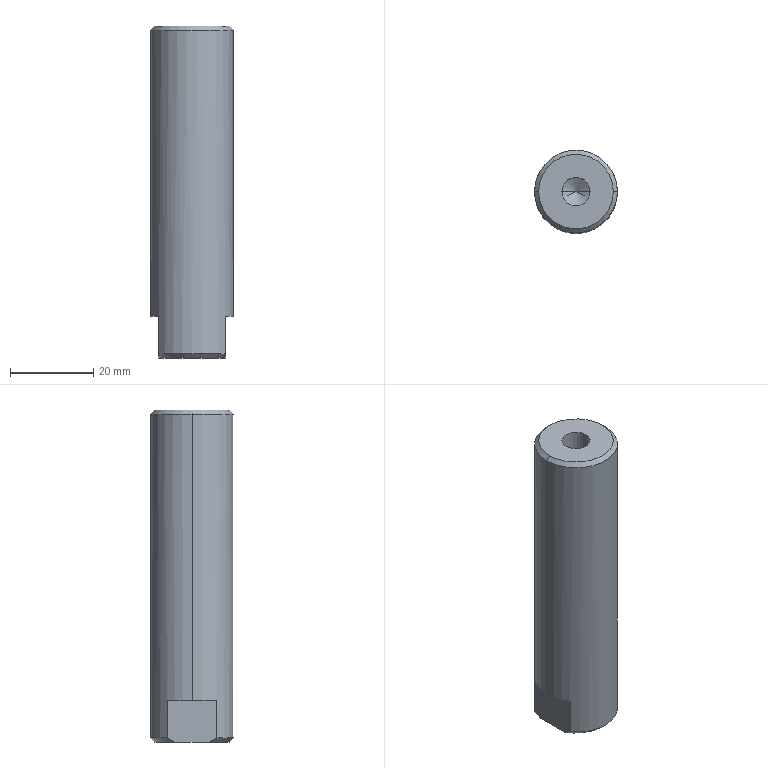Part | STEP file | 1 solid | 16 faces | box 20 x 20 x 80 mm | volume 24015 mm3 | cone 6 | plane 6 | cylinder 4 | commonest cylinder face diameters 6.8 x2 20 x2
STEP:
#1=CARTESIAN_POINT('',(0.,0.,0.));
#2=DIRECTION('',(0.,0.,1.));
#3=DIRECTION('',(1.,0.,0.));
#4=AXIS2_PLACEMENT_3D('',#1,#2,#3);
#5=CARTESIAN_POINT('',(3.4,0.,60.25));
#6=VERTEX_POINT('',#5);
#7=CARTESIAN_POINT('',(3.4,0.,80.));
#8=VERTEX_POINT('',#7);
#9=CARTESIAN_POINT('',(3.4,0.,80.));
#10=DIRECTION('',(0.,0.,1.));
#11=VECTOR('',#10,1.);
#12=LINE('',#9,#11);
#13=CARTESIAN_POINT('',(0.,0.,80.));
#14=DIRECTION('',(0.,0.,1.));
#15=DIRECTION('',(1.,0.,0.));
#16=AXIS2_PLACEMENT_3D('',#13,#14,#15);
#17=CYLINDRICAL_SURFACE('',#16,3.4);
#18=CARTESIAN_POINT('',(6.283,0.));
#19=DIRECTION('',(0.,1.));
#20=VECTOR('',#19,1.);
#21=LINE('',#18,#20);
#22=(GEOMETRIC_REPRESENTATION_CONTEXT(2)PARAMETRIC_REPRESENTATION_CONTEXT()REPRESENTATION_CONTEXT('',''));
#23=DEFINITIONAL_REPRESENTATION('',(#21),#22);
#24=PCURVE('',#17,#23);
#25=CARTESIAN_POINT('',(0.,0.,80.));
#26=DIRECTION('',(0.,0.,1.));
#27=DIRECTION('',(1.,0.,0.));
#28=AXIS2_PLACEMENT_3D('',#25,#26,#27);
#29=CYLINDRICAL_SURFACE('',#28,3.4);
#30=CARTESIAN_POINT('',(0.,0.));
#31=DIRECTION('',(0.,1.));
#32=VECTOR('',#31,1.);
#33=LINE('',#30,#32);
#34=(GEOMETRIC_REPRESENTATION_CONTEXT(2)PARAMETRIC_REPRESENTATION_CONTEXT()REPRESENTATION_CONTEXT('',''));
#35=DEFINITIONAL_REPRESENTATION('',(#33),#34);
#36=PCURVE('',#29,#35);
#37=SURFACE_CURVE('',#12,(#24,#36),.PCURVE_S1.);
#38=EDGE_CURVE('',#6,#8,#37,.T.);
#39=ORIENTED_EDGE('',*,*,#38,.T.);
#40=CARTESIAN_POINT('',(-3.4,0.,80.));
#41=VERTEX_POINT('',#40);
#42=CARTESIAN_POINT('',(0.,0.,80.));
#43=DIRECTION('',(0.,0.,1.));
#44=DIRECTION('',(1.,0.,0.));
#45=AXIS2_PLACEMENT_3D('',#42,#43,#44);
#46=CIRCLE('',#45,3.4);
#47=CARTESIAN_POINT('',(0.,0.));
#48=DIRECTION('',(1.,0.));
#49=VECTOR('',#48,1.);
#50=LINE('',#47,#49);
#51=(GEOMETRIC_REPRESENTATION_CONTEXT(2)PARAMETRIC_REPRESENTATION_CONTEXT()REPRESENTATION_CONTEXT('',''));
#52=DEFINITIONAL_REPRESENTATION('',(#50),#51);
#53=PCURVE('',#17,#52);
#54=CARTESIAN_POINT('',(0.,0.,80.));
#55=DIRECTION('',(0.,0.,1.));
#56=DIRECTION('',(1.,0.,0.));
#57=AXIS2_PLACEMENT_3D('',#54,#55,#56);
#58=PLANE('',#57);
#59=CARTESIAN_POINT('',(0.,0.));
#60=DIRECTION('',(1.,0.));
#61=AXIS2_PLACEMENT_2D('',#59,#60);
#62=CIRCLE('',#61,3.4);
#63=(GEOMETRIC_REPRESENTATION_CONTEXT(2)PARAMETRIC_REPRESENTATION_CONTEXT()REPRESENTATION_CONTEXT('',''));
#64=DEFINITIONAL_REPRESENTATION('',(#62),#63);
#65=PCURVE('',#58,#64);
#66=SURFACE_CURVE('',#46,(#53,#65),.PCURVE_S1.);
#67=EDGE_CURVE('',#41,#8,#66,.T.);
#68=ORIENTED_EDGE('',*,*,#67,.F.);
#69=CARTESIAN_POINT('',(-3.4,0.,60.25));
#70=VERTEX_POINT('',#69);
#71=CARTESIAN_POINT('',(-3.4,0.,80.));
#72=DIRECTION('',(0.,0.,1.));
#73=VECTOR('',#72,1.);
#74=LINE('',#71,#73);
#75=CARTESIAN_POINT('',(3.142,0.));
#76=DIRECTION('',(0.,1.));
#77=VECTOR('',#76,1.);
#78=LINE('',#75,#77);
#79=(GEOMETRIC_REPRESENTATION_CONTEXT(2)PARAMETRIC_REPRESENTATION_CONTEXT()REPRESENTATION_CONTEXT('',''));
#80=DEFINITIONAL_REPRESENTATION('',(#78),#79);
#81=PCURVE('',#17,#80);
#82=CARTESIAN_POINT('',(3.142,0.));
#83=DIRECTION('',(0.,1.));
#84=VECTOR('',#83,1.);
#85=LINE('',#82,#84);
#86=(GEOMETRIC_REPRESENTATION_CONTEXT(2)PARAMETRIC_REPRESENTATION_CONTEXT()REPRESENTATION_CONTEXT('',''));
#87=DEFINITIONAL_REPRESENTATION('',(#85),#86);
#88=PCURVE('',#29,#87);
#89=SURFACE_CURVE('',#74,(#81,#88),.PCURVE_S1.);
#90=EDGE_CURVE('',#70,#41,#89,.T.);
#91=ORIENTED_EDGE('',*,*,#90,.F.);
#92=CARTESIAN_POINT('',(0.,0.,60.25));
#93=DIRECTION('',(0.,0.,1.));
#94=DIRECTION('',(1.,0.,0.));
#95=AXIS2_PLACEMENT_3D('',#92,#93,#94);
#96=CIRCLE('',#95,3.4);
#97=CARTESIAN_POINT('',(0.,-19.75));
#98=DIRECTION('',(1.,0.));
#99=VECTOR('',#98,1.);
#100=LINE('',#97,#99);
#101=(GEOMETRIC_REPRESENTATION_CONTEXT(2)PARAMETRIC_REPRESENTATION_CONTEXT()REPRESENTATION_CONTEXT('',''));
#102=DEFINITIONAL_REPRESENTATION('',(#100),#101);
#103=PCURVE('',#17,#102);
#104=CARTESIAN_POINT('',(0.,0.,60.25));
#105=DIRECTION('',(0.,0.,1.));
#106=DIRECTION('',(1.,0.,0.));
#107=AXIS2_PLACEMENT_3D('',#104,#105,#106);
#108=CONICAL_SURFACE('',#107,3.4,1.03);
#109=CARTESIAN_POINT('',(0.,0.));
#110=DIRECTION('',(1.,0.));
#111=VECTOR('',#110,1.);
#112=LINE('',#109,#111);
#113=(GEOMETRIC_REPRESENTATION_CONTEXT(2)PARAMETRIC_REPRESENTATION_CONTEXT()REPRESENTATION_CONTEXT('',''));
#114=DEFINITIONAL_REPRESENTATION('',(#112),#113);
#115=PCURVE('',#108,#114);
#116=SURFACE_CURVE('',#96,(#103,#115),.PCURVE_S1.);
#117=EDGE_CURVE('',#70,#6,#116,.T.);
#118=ORIENTED_EDGE('',*,*,#117,.T.);
#119=EDGE_LOOP('',(#39,#68,#91,#118));
#120=FACE_BOUND('',#119,.F.);
#121=ADVANCED_FACE('',(#120),#17,.F.);
#122=ORIENTED_EDGE('',*,*,#117,.F.);
#123=CARTESIAN_POINT('',(0.,0.,58.207));
#124=VERTEX_POINT('',#123);
#125=CARTESIAN_POINT('',(-3.4,0.,60.25));
#126=DIRECTION('',(-0.8572,0.,0.515));
#127=VECTOR('',#126,1.);
#128=LINE('',#125,#127);
#129=CARTESIAN_POINT('',(3.142,0.));
#130=DIRECTION('',(0.,1.));
#131=VECTOR('',#130,1.);
#132=LINE('',#129,#131);
#133=(GEOMETRIC_REPRESENTATION_CONTEXT(2)PARAMETRIC_REPRESENTATION_CONTEXT()REPRESENTATION_CONTEXT('',''));
#134=DEFINITIONAL_REPRESENTATION('',(#132),#133);
#135=PCURVE('',#108,#134);
#136=CARTESIAN_POINT('',(0.,0.,60.25));
#137=DIRECTION('',(0.,0.,1.));
#138=DIRECTION('',(1.,0.,0.));
#139=AXIS2_PLACEMENT_3D('',#136,#137,#138);
#140=CONICAL_SURFACE('',#139,3.4,1.03);
#141=CARTESIAN_POINT('',(3.142,0.));
#142=DIRECTION('',(0.,1.));
#143=VECTOR('',#142,1.);
#144=LINE('',#141,#143);
#145=(GEOMETRIC_REPRESENTATION_CONTEXT(2)PARAMETRIC_REPRESENTATION_CONTEXT()REPRESENTATION_CONTEXT('',''));
#146=DEFINITIONAL_REPRESENTATION('',(#144),#145);
#147=PCURVE('',#140,#146);
#148=SURFACE_CURVE('',#128,(#135,#147),.PCURVE_S1.);
#149=EDGE_CURVE('',#124,#70,#148,.T.);
#150=ORIENTED_EDGE('',*,*,#149,.F.);
#151=CARTESIAN_POINT('',(3.4,0.,60.25));
#152=DIRECTION('',(0.8572,0.,0.515));
#153=VECTOR('',#152,1.);
#154=LINE('',#151,#153);
#155=CARTESIAN_POINT('',(6.283,0.));
#156=DIRECTION('',(0.,1.));
#157=VECTOR('',#156,1.);
#158=LINE('',#155,#157);
#159=(GEOMETRIC_REPRESENTATION_CONTEXT(2)PARAMETRIC_REPRESENTATION_CONTEXT()REPRESENTATION_CONTEXT('',''));
#160=DEFINITIONAL_REPRESENTATION('',(#158),#159);
#161=PCURVE('',#108,#160);
#162=CARTESIAN_POINT('',(0.,0.));
#163=DIRECTION('',(0.,1.));
#164=VECTOR('',#163,1.);
#165=LINE('',#162,#164);
#166=(GEOMETRIC_REPRESENTATION_CONTEXT(2)PARAMETRIC_REPRESENTATION_CONTEXT()REPRESENTATION_CONTEXT('',''));
#167=DEFINITIONAL_REPRESENTATION('',(#165),#166);
#168=PCURVE('',#140,#167);
#169=SURFACE_CURVE('',#154,(#161,#168),.PCURVE_S1.);
#170=EDGE_CURVE('',#124,#6,#169,.T.);
#171=ORIENTED_EDGE('',*,*,#170,.T.);
#172=EDGE_LOOP('',(#122,#150,#171));
#173=FACE_BOUND('',#172,.F.);
#174=ADVANCED_FACE('',(#173),#108,.F.);
#175=CARTESIAN_POINT('',(9.,0.,80.));
#176=VERTEX_POINT('',#175);
#177=CARTESIAN_POINT('',(-9.,0.,80.));
#178=VERTEX_POINT('',#177);
#179=CARTESIAN_POINT('',(0.,0.,80.));
#180=DIRECTION('',(0.,0.,1.));
#181=DIRECTION('',(1.,0.,0.));
#182=AXIS2_PLACEMENT_3D('',#179,#180,#181);
#183=CIRCLE('',#182,9.);
#184=CARTESIAN_POINT('',(0.,0.,80.));
#185=DIRECTION('',(0.,0.,-1.));
#186=DIRECTION('',(-1.,0.,0.));
#187=AXIS2_PLACEMENT_3D('',#184,#185,#186);
#188=CONICAL_SURFACE('',#187,9.,0.7854);
#189=CARTESIAN_POINT('',(3.142,0.));
#190=DIRECTION('',(-1.,0.));
#191=VECTOR('',#190,1.);
#192=LINE('',#189,#191);
#193=(GEOMETRIC_REPRESENTATION_CONTEXT(2)PARAMETRIC_REPRESENTATION_CONTEXT()REPRESENTATION_CONTEXT('',''));
#194=DEFINITIONAL_REPRESENTATION('',(#192),#193);
#195=PCURVE('',#188,#194);
#196=CARTESIAN_POINT('',(0.,0.));
#197=DIRECTION('',(1.,0.));
#198=AXIS2_PLACEMENT_2D('',#196,#197);
#199=CIRCLE('',#198,9.);
#200=(GEOMETRIC_REPRESENTATION_CONTEXT(2)PARAMETRIC_REPRESENTATION_CONTEXT()REPRESENTATION_CONTEXT('',''));
#201=DEFINITIONAL_REPRESENTATION('',(#199),#200);
#202=PCURVE('',#58,#201);
#203=SURFACE_CURVE('',#183,(#195,#202),.PCURVE_S1.);
#204=EDGE_CURVE('',#176,#178,#203,.T.);
#205=ORIENTED_EDGE('',*,*,#204,.F.);
#206=CARTESIAN_POINT('',(10.,0.,79.));
#207=VERTEX_POINT('',#206);
#208=CARTESIAN_POINT('',(9.,0.,80.));
#209=DIRECTION('',(0.7071,0.,-0.7071));
#210=VECTOR('',#209,1.);
#211=LINE('',#208,#210);
#212=CARTESIAN_POINT('',(3.142,0.));
#213=DIRECTION('',(0.,1.));
#214=VECTOR('',#213,1.);
#215=LINE('',#212,#214);
#216=(GEOMETRIC_REPRESENTATION_CONTEXT(2)PARAMETRIC_REPRESENTATION_CONTEXT()REPRESENTATION_CONTEXT('',''));
#217=DEFINITIONAL_REPRESENTATION('',(#215),#216);
#218=PCURVE('',#188,#217);
#219=CARTESIAN_POINT('',(0.,0.,80.));
#220=DIRECTION('',(0.,0.,-1.));
#221=DIRECTION('',(-1.,0.,0.));
#222=AXIS2_PLACEMENT_3D('',#219,#220,#221);
#223=CONICAL_SURFACE('',#222,9.,0.7854);
#224=CARTESIAN_POINT('',(3.142,0.));
#225=DIRECTION('',(0.,1.));
#226=VECTOR('',#225,1.);
#227=LINE('',#224,#226);
#228=(GEOMETRIC_REPRESENTATION_CONTEXT(2)PARAMETRIC_REPRESENTATION_CONTEXT()REPRESENTATION_CONTEXT('',''));
#229=DEFINITIONAL_REPRESENTATION('',(#227),#228);
#230=PCURVE('',#223,#229);
#231=SURFACE_CURVE('',#211,(#218,#230),.PCURVE_S1.);
#232=EDGE_CURVE('',#176,#207,#231,.T.);
#233=ORIENTED_EDGE('',*,*,#232,.T.);
#234=CARTESIAN_POINT('',(-10.,0.,79.));
#235=VERTEX_POINT('',#234);
#236=CARTESIAN_POINT('',(0.,0.,79.));
#237=DIRECTION('',(0.,0.,-1.));
#238=DIRECTION('',(1.,0.,0.));
#239=AXIS2_PLACEMENT_3D('',#236,#237,#238);
#240=CIRCLE('',#239,10.);
#241=CARTESIAN_POINT('',(-3.142,1.));
#242=DIRECTION('',(1.,0.));
#243=VECTOR('',#242,1.);
#244=LINE('',#241,#243);
#245=(GEOMETRIC_REPRESENTATION_CONTEXT(2)PARAMETRIC_REPRESENTATION_CONTEXT()REPRESENTATION_CONTEXT('',''));
#246=DEFINITIONAL_REPRESENTATION('',(#244),#245);
#247=PCURVE('',#188,#246);
#248=CARTESIAN_POINT('',(0.,0.,80.));
#249=DIRECTION('',(0.,0.,-1.));
#250=DIRECTION('',(-1.,0.,0.));
#251=AXIS2_PLACEMENT_3D('',#248,#249,#250);
#252=CYLINDRICAL_SURFACE('',#251,10.);
#253=CARTESIAN_POINT('',(-3.142,1.));
#254=DIRECTION('',(1.,0.));
#255=VECTOR('',#254,1.);
#256=LINE('',#253,#255);
#257=(GEOMETRIC_REPRESENTATION_CONTEXT(2)PARAMETRIC_REPRESENTATION_CONTEXT()REPRESENTATION_CONTEXT('',''));
#258=DEFINITIONAL_REPRESENTATION('',(#256),#257);
#259=PCURVE('',#252,#258);
#260=SURFACE_CURVE('',#240,(#247,#259),.PCURVE_S1.);
#261=EDGE_CURVE('',#235,#207,#260,.T.);
#262=ORIENTED_EDGE('',*,*,#261,.F.);
#263=CARTESIAN_POINT('',(-9.,0.,80.));
#264=DIRECTION('',(-0.7071,0.,-0.7071));
#265=VECTOR('',#264,1.);
#266=LINE('',#263,#265);
#267=CARTESIAN_POINT('',(0.,0.));
#268=DIRECTION('',(0.,1.));
#269=VECTOR('',#268,1.);
#270=LINE('',#267,#269);
#271=(GEOMETRIC_REPRESENTATION_CONTEXT(2)PARAMETRIC_REPRESENTATION_CONTEXT()REPRESENTATION_CONTEXT('',''));
#272=DEFINITIONAL_REPRESENTATION('',(#270),#271);
#273=PCURVE('',#188,#272);
#274=CARTESIAN_POINT('',(6.283,0.));
#275=DIRECTION('',(0.,1.));
#276=VECTOR('',#275,1.);
#277=LINE('',#274,#276);
#278=(GEOMETRIC_REPRESENTATION_CONTEXT(2)PARAMETRIC_REPRESENTATION_CONTEXT()REPRESENTATION_CONTEXT('',''));
#279=DEFINITIONAL_REPRESENTATION('',(#277),#278);
#280=PCURVE('',#223,#279);
#281=SURFACE_CURVE('',#266,(#273,#280),.PCURVE_S1.);
#282=EDGE_CURVE('',#178,#235,#281,.T.);
#283=ORIENTED_EDGE('',*,*,#282,.F.);
#284=EDGE_LOOP('',(#205,#233,#262,#283));
#285=FACE_BOUND('',#284,.T.);
#286=ADVANCED_FACE('',(#285),#188,.T.);
#287=ORIENTED_EDGE('',*,*,#261,.T.);
#288=CARTESIAN_POINT('',(10.,0.,10.));
#289=VERTEX_POINT('',#288);
#290=CARTESIAN_POINT('',(10.,0.,80.));
#291=DIRECTION('',(0.,0.,-1.));
#292=VECTOR('',#291,1.);
#293=LINE('',#290,#292);
#294=CARTESIAN_POINT('',(3.142,0.));
#295=DIRECTION('',(0.,1.));
#296=VECTOR('',#295,1.);
#297=LINE('',#294,#296);
#298=(GEOMETRIC_REPRESENTATION_CONTEXT(2)PARAMETRIC_REPRESENTATION_CONTEXT()REPRESENTATION_CONTEXT('',''));
#299=DEFINITIONAL_REPRESENTATION('',(#297),#298);
#300=PCURVE('',#252,#299);
#301=CARTESIAN_POINT('',(0.,0.,80.));
#302=DIRECTION('',(0.,0.,-1.));
#303=DIRECTION('',(-1.,0.,0.));
#304=AXIS2_PLACEMENT_3D('',#301,#302,#303);
#305=CYLINDRICAL_SURFACE('',#304,10.);
#306=CARTESIAN_POINT('',(3.142,0.));
#307=DIRECTION('',(0.,1.));
#308=VECTOR('',#307,1.);
#309=LINE('',#306,#308);
#310=(GEOMETRIC_REPRESENTATION_CONTEXT(2)PARAMETRIC_REPRESENTATION_CONTEXT()REPRESENTATION_CONTEXT('',''));
#311=DEFINITIONAL_REPRESENTATION('',(#309),#310);
#312=PCURVE('',#305,#311);
#313=SURFACE_CURVE('',#293,(#300,#312),.PCURVE_S1.);
#314=EDGE_CURVE('',#207,#289,#313,.T.);
#315=ORIENTED_EDGE('',*,*,#314,.T.);
#316=CARTESIAN_POINT('',(8.,6.,10.));
#317=VERTEX_POINT('',#316);
#318=CARTESIAN_POINT('',(0.,0.,10.));
#319=DIRECTION('',(0.,0.,-1.));
#320=DIRECTION('',(-1.,0.,0.));
#321=AXIS2_PLACEMENT_3D('',#318,#319,#320);
#322=CIRCLE('',#321,10.);
#323=CARTESIAN_POINT('',(0.,70.));
#324=DIRECTION('',(1.,0.));
#325=VECTOR('',#324,1.);
#326=LINE('',#323,#325);
#327=(GEOMETRIC_REPRESENTATION_CONTEXT(2)PARAMETRIC_REPRESENTATION_CONTEXT()REPRESENTATION_CONTEXT('',''));
#328=DEFINITIONAL_REPRESENTATION('',(#326),#327);
#329=PCURVE('',#252,#328);
#330=CARTESIAN_POINT('',(0.,0.,10.));
#331=DIRECTION('',(0.,0.,-1.));
#332=DIRECTION('',(-1.,0.,0.));
#333=AXIS2_PLACEMENT_3D('',#330,#331,#332);
#334=PLANE('',#333);
#335=CARTESIAN_POINT('',(0.,0.));
#336=DIRECTION('',(1.,0.));
#337=AXIS2_PLACEMENT_2D('',#335,#336);
#338=CIRCLE('',#337,10.);
#339=(GEOMETRIC_REPRESENTATION_CONTEXT(2)PARAMETRIC_REPRESENTATION_CONTEXT()REPRESENTATION_CONTEXT('',''));
#340=DEFINITIONAL_REPRESENTATION('',(#338),#339);
#341=PCURVE('',#334,#340);
#342=SURFACE_CURVE('',#322,(#329,#341),.PCURVE_S1.);
#343=EDGE_CURVE('',#317,#289,#342,.T.);
#344=ORIENTED_EDGE('',*,*,#343,.F.);
#345=CARTESIAN_POINT('',(8.,6.,1.));
#346=VERTEX_POINT('',#345);
#347=CARTESIAN_POINT('',(8.,6.,10.));
#348=DIRECTION('',(0.,0.,-1.));
#349=VECTOR('',#348,1.);
#350=LINE('',#347,#349);
#351=CARTESIAN_POINT('',(2.498,70.));
#352=DIRECTION('',(0.,1.));
#353=VECTOR('',#352,1.);
#354=LINE('',#351,#353);
#355=(GEOMETRIC_REPRESENTATION_CONTEXT(2)PARAMETRIC_REPRESENTATION_CONTEXT()REPRESENTATION_CONTEXT('',''));
#356=DEFINITIONAL_REPRESENTATION('',(#354),#355);
#357=PCURVE('',#252,#356);
#358=CARTESIAN_POINT('',(8.,0.,10.));
#359=DIRECTION('',(1.,0.,0.));
#360=DIRECTION('',(0.,0.,-1.));
#361=AXIS2_PLACEMENT_3D('',#358,#359,#360);
#362=PLANE('',#361);
#363=CARTESIAN_POINT('',(0.,6.));
#364=DIRECTION('',(1.,0.));
#365=VECTOR('',#364,1.);
#366=LINE('',#363,#365);
#367=(GEOMETRIC_REPRESENTATION_CONTEXT(2)PARAMETRIC_REPRESENTATION_CONTEXT()REPRESENTATION_CONTEXT('',''));
#368=DEFINITIONAL_REPRESENTATION('',(#366),#367);
#369=PCURVE('',#362,#368);
#370=SURFACE_CURVE('',#350,(#357,#369),.PCURVE_S1.);
#371=EDGE_CURVE('',#317,#346,#370,.T.);
#372=ORIENTED_EDGE('',*,*,#371,.T.);
#373=CARTESIAN_POINT('',(-8.,6.,1.));
#374=VERTEX_POINT('',#373);
#375=CARTESIAN_POINT('',(0.,0.,1.));
#376=DIRECTION('',(0.,0.,1.));
#377=DIRECTION('',(1.,0.,0.));
#378=AXIS2_PLACEMENT_3D('',#375,#376,#377);
#379=CIRCLE('',#378,10.);
#380=CARTESIAN_POINT('',(3.142,79.));
#381=DIRECTION('',(-1.,0.));
#382=VECTOR('',#381,1.);
#383=LINE('',#380,#382);
#384=(GEOMETRIC_REPRESENTATION_CONTEXT(2)PARAMETRIC_REPRESENTATION_CONTEXT()REPRESENTATION_CONTEXT('',''));
#385=DEFINITIONAL_REPRESENTATION('',(#383),#384);
#386=PCURVE('',#252,#385);
#387=CARTESIAN_POINT('',(0.,0.,1.));
#388=DIRECTION('',(0.,0.,1.));
#389=DIRECTION('',(1.,0.,0.));
#390=AXIS2_PLACEMENT_3D('',#387,#388,#389);
#391=CONICAL_SURFACE('',#390,10.,0.7854);
#392=CARTESIAN_POINT('',(0.,0.));
#393=DIRECTION('',(1.,0.));
#394=VECTOR('',#393,1.);
#395=LINE('',#392,#394);
#396=(GEOMETRIC_REPRESENTATION_CONTEXT(2)PARAMETRIC_REPRESENTATION_CONTEXT()REPRESENTATION_CONTEXT('',''));
#397=DEFINITIONAL_REPRESENTATION('',(#395),#396);
#398=PCURVE('',#391,#397);
#399=SURFACE_CURVE('',#379,(#386,#398),.PCURVE_S1.);
#400=EDGE_CURVE('',#346,#374,#399,.T.);
#401=ORIENTED_EDGE('',*,*,#400,.T.);
#402=CARTESIAN_POINT('',(-8.,6.,10.));
#403=VERTEX_POINT('',#402);
#404=CARTESIAN_POINT('',(-8.,6.,10.));
#405=DIRECTION('',(0.,0.,-1.));
#406=VECTOR('',#405,1.);
#407=LINE('',#404,#406);
#408=CARTESIAN_POINT('',(0.6435,70.));
#409=DIRECTION('',(0.,1.));
#410=VECTOR('',#409,1.);
#411=LINE('',#408,#410);
#412=(GEOMETRIC_REPRESENTATION_CONTEXT(2)PARAMETRIC_REPRESENTATION_CONTEXT()REPRESENTATION_CONTEXT('',''));
#413=DEFINITIONAL_REPRESENTATION('',(#411),#412);
#414=PCURVE('',#252,#413);
#415=CARTESIAN_POINT('',(-8.,0.,10.));
#416=DIRECTION('',(1.,0.,0.));
#417=DIRECTION('',(0.,0.,-1.));
#418=AXIS2_PLACEMENT_3D('',#415,#416,#417);
#419=PLANE('',#418);
#420=CARTESIAN_POINT('',(0.,6.));
#421=DIRECTION('',(1.,0.));
#422=VECTOR('',#421,1.);
#423=LINE('',#420,#422);
#424=(GEOMETRIC_REPRESENTATION_CONTEXT(2)PARAMETRIC_REPRESENTATION_CONTEXT()REPRESENTATION_CONTEXT('',''));
#425=DEFINITIONAL_REPRESENTATION('',(#423),#424);
#426=PCURVE('',#419,#425);
#427=SURFACE_CURVE('',#407,(#414,#426),.PCURVE_S1.);
#428=EDGE_CURVE('',#403,#374,#427,.T.);
#429=ORIENTED_EDGE('',*,*,#428,.F.);
#430=CARTESIAN_POINT('',(-10.,0.,10.));
#431=VERTEX_POINT('',#430);
#432=CARTESIAN_POINT('',(0.,0.,10.));
#433=DIRECTION('',(0.,0.,-1.));
#434=DIRECTION('',(-1.,0.,0.));
#435=AXIS2_PLACEMENT_3D('',#432,#433,#434);
#436=CIRCLE('',#435,10.);
#437=CARTESIAN_POINT('',(0.,70.));
#438=DIRECTION('',(1.,0.));
#439=VECTOR('',#438,1.);
#440=LINE('',#437,#439);
#441=(GEOMETRIC_REPRESENTATION_CONTEXT(2)PARAMETRIC_REPRESENTATION_CONTEXT()REPRESENTATION_CONTEXT('',''));
#442=DEFINITIONAL_REPRESENTATION('',(#440),#441);
#443=PCURVE('',#252,#442);
#444=CARTESIAN_POINT('',(0.,0.,10.));
#445=DIRECTION('',(0.,0.,-1.));
#446=DIRECTION('',(-1.,0.,0.));
#447=AXIS2_PLACEMENT_3D('',#444,#445,#446);
#448=PLANE('',#447);
#449=CARTESIAN_POINT('',(0.,0.));
#450=DIRECTION('',(1.,0.));
#451=AXIS2_PLACEMENT_2D('',#449,#450);
#452=CIRCLE('',#451,10.);
#453=(GEOMETRIC_REPRESENTATION_CONTEXT(2)PARAMETRIC_REPRESENTATION_CONTEXT()REPRESENTATION_CONTEXT('',''));
#454=DEFINITIONAL_REPRESENTATION('',(#452),#453);
#455=PCURVE('',#448,#454);
#456=SURFACE_CURVE('',#436,(#443,#455),.PCURVE_S1.);
#457=EDGE_CURVE('',#431,#403,#456,.T.);
#458=ORIENTED_EDGE('',*,*,#457,.F.);
#459=CARTESIAN_POINT('',(-10.,0.,80.));
#460=DIRECTION('',(0.,0.,-1.));
#461=VECTOR('',#460,1.);
#462=LINE('',#459,#461);
#463=CARTESIAN_POINT('',(0.,0.));
#464=DIRECTION('',(0.,1.));
#465=VECTOR('',#464,1.);
#466=LINE('',#463,#465);
#467=(GEOMETRIC_REPRESENTATION_CONTEXT(2)PARAMETRIC_REPRESENTATION_CONTEXT()REPRESENTATION_CONTEXT('',''));
#468=DEFINITIONAL_REPRESENTATION('',(#466),#467);
#469=PCURVE('',#252,#468);
#470=CARTESIAN_POINT('',(6.283,0.));
#471=DIRECTION('',(0.,1.));
#472=VECTOR('',#471,1.);
#473=LINE('',#470,#472);
#474=(GEOMETRIC_REPRESENTATION_CONTEXT(2)PARAMETRIC_REPRESENTATION_CONTEXT()REPRESENTATION_CONTEXT('',''));
#475=DEFINITIONAL_REPRESENTATION('',(#473),#474);
#476=PCURVE('',#305,#475);
#477=SURFACE_CURVE('',#462,(#469,#476),.PCURVE_S1.);
#478=EDGE_CURVE('',#235,#431,#477,.T.);
#479=ORIENTED_EDGE('',*,*,#478,.F.);
#480=EDGE_LOOP('',(#287,#315,#344,#372,#401,#429,#458,#479));
#481=FACE_BOUND('',#480,.T.);
#482=ADVANCED_FACE('',(#481),#252,.T.);
#483=ORIENTED_EDGE('',*,*,#314,.F.);
#484=CARTESIAN_POINT('',(0.,0.,79.));
#485=DIRECTION('',(0.,0.,-1.));
#486=DIRECTION('',(1.,0.,0.));
#487=AXIS2_PLACEMENT_3D('',#484,#485,#486);
#488=CIRCLE('',#487,10.);
#489=CARTESIAN_POINT('',(3.142,1.));
#490=DIRECTION('',(1.,0.));
#491=VECTOR('',#490,1.);
#492=LINE('',#489,#491);
#493=(GEOMETRIC_REPRESENTATION_CONTEXT(2)PARAMETRIC_REPRESENTATION_CONTEXT()REPRESENTATION_CONTEXT('',''));
#494=DEFINITIONAL_REPRESENTATION('',(#492),#493);
#495=PCURVE('',#305,#494);
#496=CARTESIAN_POINT('',(3.142,1.));
#497=DIRECTION('',(1.,0.));
#498=VECTOR('',#497,1.);
#499=LINE('',#496,#498);
#500=(GEOMETRIC_REPRESENTATION_CONTEXT(2)PARAMETRIC_REPRESENTATION_CONTEXT()REPRESENTATION_CONTEXT('',''));
#501=DEFINITIONAL_REPRESENTATION('',(#499),#500);
#502=PCURVE('',#223,#501);
#503=SURFACE_CURVE('',#488,(#495,#502),.PCURVE_S1.);
#504=EDGE_CURVE('',#207,#235,#503,.T.);
#505=ORIENTED_EDGE('',*,*,#504,.T.);
#506=ORIENTED_EDGE('',*,*,#478,.T.);
#507=CARTESIAN_POINT('',(-8.,-6.,10.));
#508=VERTEX_POINT('',#507);
#509=CARTESIAN_POINT('',(0.,0.,10.));
#510=DIRECTION('',(0.,0.,-1.));
#511=DIRECTION('',(-1.,0.,0.));
#512=AXIS2_PLACEMENT_3D('',#509,#510,#511);
#513=CIRCLE('',#512,10.);
#514=CARTESIAN_POINT('',(0.,70.));
#515=DIRECTION('',(1.,0.));
#516=VECTOR('',#515,1.);
#517=LINE('',#514,#516);
#518=(GEOMETRIC_REPRESENTATION_CONTEXT(2)PARAMETRIC_REPRESENTATION_CONTEXT()REPRESENTATION_CONTEXT('',''));
#519=DEFINITIONAL_REPRESENTATION('',(#517),#518);
#520=PCURVE('',#305,#519);
#521=CARTESIAN_POINT('',(0.,0.));
#522=DIRECTION('',(1.,0.));
#523=AXIS2_PLACEMENT_2D('',#521,#522);
#524=CIRCLE('',#523,10.);
#525=(GEOMETRIC_REPRESENTATION_CONTEXT(2)PARAMETRIC_REPRESENTATION_CONTEXT()REPRESENTATION_CONTEXT('',''));
#526=DEFINITIONAL_REPRESENTATION('',(#524),#525);
#527=PCURVE('',#448,#526);
#528=SURFACE_CURVE('',#513,(#520,#527),.PCURVE_S1.);
#529=EDGE_CURVE('',#508,#431,#528,.T.);
#530=ORIENTED_EDGE('',*,*,#529,.F.);
#531=CARTESIAN_POINT('',(-8.,-6.,1.));
#532=VERTEX_POINT('',#531);
#533=CARTESIAN_POINT('',(-8.,-6.,10.));
#534=DIRECTION('',(0.,0.,-1.));
#535=VECTOR('',#534,1.);
#536=LINE('',#533,#535);
#537=CARTESIAN_POINT('',(5.64,70.));
#538=DIRECTION('',(0.,1.));
#539=VECTOR('',#538,1.);
#540=LINE('',#537,#539);
#541=(GEOMETRIC_REPRESENTATION_CONTEXT(2)PARAMETRIC_REPRESENTATION_CONTEXT()REPRESENTATION_CONTEXT('',''));
#542=DEFINITIONAL_REPRESENTATION('',(#540),#541);
#543=PCURVE('',#305,#542);
#544=CARTESIAN_POINT('',(0.,-6.));
#545=DIRECTION('',(1.,0.));
#546=VECTOR('',#545,1.);
#547=LINE('',#544,#546);
#548=(GEOMETRIC_REPRESENTATION_CONTEXT(2)PARAMETRIC_REPRESENTATION_CONTEXT()REPRESENTATION_CONTEXT('',''));
#549=DEFINITIONAL_REPRESENTATION('',(#547),#548);
#550=PCURVE('',#419,#549);
#551=SURFACE_CURVE('',#536,(#543,#550),.PCURVE_S1.);
#552=EDGE_CURVE('',#508,#532,#551,.T.);
#553=ORIENTED_EDGE('',*,*,#552,.T.);
#554=CARTESIAN_POINT('',(8.,-6.,1.));
#555=VERTEX_POINT('',#554);
#556=CARTESIAN_POINT('',(0.,0.,1.));
#557=DIRECTION('',(0.,0.,1.));
#558=DIRECTION('',(1.,0.,0.));
#559=AXIS2_PLACEMENT_3D('',#556,#557,#558);
#560=CIRCLE('',#559,10.);
#561=CARTESIAN_POINT('',(9.425,79.));
#562=DIRECTION('',(-1.,0.));
#563=VECTOR('',#562,1.);
#564=LINE('',#561,#563);
#565=(GEOMETRIC_REPRESENTATION_CONTEXT(2)PARAMETRIC_REPRESENTATION_CONTEXT()REPRESENTATION_CONTEXT('',''));
#566=DEFINITIONAL_REPRESENTATION('',(#564),#565);
#567=PCURVE('',#305,#566);
#568=CARTESIAN_POINT('',(0.,0.,1.));
#569=DIRECTION('',(0.,0.,1.));
#570=DIRECTION('',(1.,0.,0.));
#571=AXIS2_PLACEMENT_3D('',#568,#569,#570);
#572=CONICAL_SURFACE('',#571,10.,0.7854);
#573=CARTESIAN_POINT('',(0.,0.));
#574=DIRECTION('',(1.,0.));
#575=VECTOR('',#574,1.);
#576=LINE('',#573,#575);
#577=(GEOMETRIC_REPRESENTATION_CONTEXT(2)PARAMETRIC_REPRESENTATION_CONTEXT()REPRESENTATION_CONTEXT('',''));
#578=DEFINITIONAL_REPRESENTATION('',(#576),#577);
#579=PCURVE('',#572,#578);
#580=SURFACE_CURVE('',#560,(#567,#579),.PCURVE_S1.);
#581=EDGE_CURVE('',#532,#555,#580,.T.);
#582=ORIENTED_EDGE('',*,*,#581,.T.);
#583=CARTESIAN_POINT('',(8.,-6.,10.));
#584=VERTEX_POINT('',#583);
#585=CARTESIAN_POINT('',(8.,-6.,10.));
#586=DIRECTION('',(0.,0.,-1.));
#587=VECTOR('',#586,1.);
#588=LINE('',#585,#587);
#589=CARTESIAN_POINT('',(3.785,70.));
#590=DIRECTION('',(0.,1.));
#591=VECTOR('',#590,1.);
#592=LINE('',#589,#591);
#593=(GEOMETRIC_REPRESENTATION_CONTEXT(2)PARAMETRIC_REPRESENTATION_CONTEXT()REPRESENTATION_CONTEXT('',''));
#594=DEFINITIONAL_REPRESENTATION('',(#592),#593);
#595=PCURVE('',#305,#594);
#596=CARTESIAN_POINT('',(0.,-6.));
#597=DIRECTION('',(1.,0.));
#598=VECTOR('',#597,1.);
#599=LINE('',#596,#598);
#600=(GEOMETRIC_REPRESENTATION_CONTEXT(2)PARAMETRIC_REPRESENTATION_CONTEXT()REPRESENTATION_CONTEXT('',''));
#601=DEFINITIONAL_REPRESENTATION('',(#599),#600);
#602=PCURVE('',#362,#601);
#603=SURFACE_CURVE('',#588,(#595,#602),.PCURVE_S1.);
#604=EDGE_CURVE('',#584,#555,#603,.T.);
#605=ORIENTED_EDGE('',*,*,#604,.F.);
#606=CARTESIAN_POINT('',(0.,0.,10.));
#607=DIRECTION('',(0.,0.,-1.));
#608=DIRECTION('',(-1.,0.,0.));
#609=AXIS2_PLACEMENT_3D('',#606,#607,#608);
#610=CIRCLE('',#609,10.);
#611=CARTESIAN_POINT('',(0.,70.));
#612=DIRECTION('',(1.,0.));
#613=VECTOR('',#612,1.);
#614=LINE('',#611,#613);
#615=(GEOMETRIC_REPRESENTATION_CONTEXT(2)PARAMETRIC_REPRESENTATION_CONTEXT()REPRESENTATION_CONTEXT('',''));
#616=DEFINITIONAL_REPRESENTATION('',(#614),#615);
#617=PCURVE('',#305,#616);
#618=CARTESIAN_POINT('',(0.,0.));
#619=DIRECTION('',(1.,0.));
#620=AXIS2_PLACEMENT_2D('',#618,#619);
#621=CIRCLE('',#620,10.);
#622=(GEOMETRIC_REPRESENTATION_CONTEXT(2)PARAMETRIC_REPRESENTATION_CONTEXT()REPRESENTATION_CONTEXT('',''));
#623=DEFINITIONAL_REPRESENTATION('',(#621),#622);
#624=PCURVE('',#334,#623);
#625=SURFACE_CURVE('',#610,(#617,#624),.PCURVE_S1.);
#626=EDGE_CURVE('',#289,#584,#625,.T.);
#627=ORIENTED_EDGE('',*,*,#626,.F.);
#628=EDGE_LOOP('',(#483,#505,#506,#530,#553,#582,#605,#627));
#629=FACE_BOUND('',#628,.T.);
#630=ADVANCED_FACE('',(#629),#305,.T.);
#631=CARTESIAN_POINT('',(8.,4.123,0.));
#632=VERTEX_POINT('',#631);
#633=CARTESIAN_POINT('',(8.,-4.123,0.));
#634=VERTEX_POINT('',#633);
#635=CARTESIAN_POINT('',(8.,0.,0.));
#636=DIRECTION('',(0.,-1.,0.));
#637=VECTOR('',#636,1.);
#638=LINE('',#635,#637);
#639=CARTESIAN_POINT('',(0.,0.,0.));
#640=DIRECTION('',(0.,0.,1.));
#641=DIRECTION('',(1.,0.,0.));
#642=AXIS2_PLACEMENT_3D('',#639,#640,#641);
#643=PLANE('',#642);
#644=CARTESIAN_POINT('',(8.,0.));
#645=DIRECTION('',(0.,-1.));
#646=VECTOR('',#645,1.);
#647=LINE('',#644,#646);
#648=(GEOMETRIC_REPRESENTATION_CONTEXT(2)PARAMETRIC_REPRESENTATION_CONTEXT()REPRESENTATION_CONTEXT('',''));
#649=DEFINITIONAL_REPRESENTATION('',(#647),#648);
#650=PCURVE('',#643,#649);
#651=CARTESIAN_POINT('',(10.,0.));
#652=DIRECTION('',(0.,-1.));
#653=VECTOR('',#652,1.);
#654=LINE('',#651,#653);
#655=(GEOMETRIC_REPRESENTATION_CONTEXT(2)PARAMETRIC_REPRESENTATION_CONTEXT()REPRESENTATION_CONTEXT('',''));
#656=DEFINITIONAL_REPRESENTATION('',(#654),#655);
#657=PCURVE('',#362,#656);
#658=SURFACE_CURVE('',#638,(#650,#657),.PCURVE_S1.);
#659=EDGE_CURVE('',#632,#634,#658,.T.);
#660=ORIENTED_EDGE('',*,*,#659,.T.);
#661=CARTESIAN_POINT('',(-8.,-4.123,0.));
#662=VERTEX_POINT('',#661);
#663=CARTESIAN_POINT('',(0.,0.,0.));
#664=DIRECTION('',(0.,0.,-1.));
#665=DIRECTION('',(1.,0.,0.));
#666=AXIS2_PLACEMENT_3D('',#663,#664,#665);
#667=CIRCLE('',#666,9.);
#668=CARTESIAN_POINT('',(9.,0.));
#669=CARTESIAN_POINT('',(9.,-15.588));
#670=CARTESIAN_POINT('',(-4.5,-7.794));
#671=CARTESIAN_POINT('',(-18.,0.));
#672=CARTESIAN_POINT('',(-4.5,7.794));
#673=CARTESIAN_POINT('',(9.,15.588));
#674=CARTESIAN_POINT('',(9.,0.));
#675=(BOUNDED_CURVE()B_SPLINE_CURVE(2,(#668,#669,#670,#671,#672,#673,#674),.UNSPECIFIED.,.T.,.F.)B_SPLINE_CURVE_WITH_KNOTS((1,2,2,2,2,1),(-2.094,0.,2.094,4.189,6.283,8.378),.UNSPECIFIED.)CURVE()GEOMETRIC_REPRESENTATION_ITEM()RATIONAL_B_SPLINE_CURVE((1.,0.5,1.,0.5,1.,0.5,1.))REPRESENTATION_ITEM(''));
#676=(GEOMETRIC_REPRESENTATION_CONTEXT(2)PARAMETRIC_REPRESENTATION_CONTEXT()REPRESENTATION_CONTEXT('',''));
#677=DEFINITIONAL_REPRESENTATION('',(#675),#676);
#678=PCURVE('',#643,#677);
#679=CARTESIAN_POINT('',(6.283,-1.));
#680=DIRECTION('',(-1.,0.));
#681=VECTOR('',#680,1.);
#682=LINE('',#679,#681);
#683=(GEOMETRIC_REPRESENTATION_CONTEXT(2)PARAMETRIC_REPRESENTATION_CONTEXT()REPRESENTATION_CONTEXT('',''));
#684=DEFINITIONAL_REPRESENTATION('',(#682),#683);
#685=PCURVE('',#572,#684);
#686=SURFACE_CURVE('',#667,(#678,#685),.PCURVE_S1.);
#687=EDGE_CURVE('',#634,#662,#686,.T.);
#688=ORIENTED_EDGE('',*,*,#687,.T.);
#689=CARTESIAN_POINT('',(-8.,4.123,0.));
#690=VERTEX_POINT('',#689);
#691=CARTESIAN_POINT('',(-8.,0.,0.));
#692=DIRECTION('',(0.,-1.,0.));
#693=VECTOR('',#692,1.);
#694=LINE('',#691,#693);
#695=CARTESIAN_POINT('',(-8.,0.));
#696=DIRECTION('',(0.,-1.));
#697=VECTOR('',#696,1.);
#698=LINE('',#695,#697);
#699=(GEOMETRIC_REPRESENTATION_CONTEXT(2)PARAMETRIC_REPRESENTATION_CONTEXT()REPRESENTATION_CONTEXT('',''));
#700=DEFINITIONAL_REPRESENTATION('',(#698),#699);
#701=PCURVE('',#643,#700);
#702=CARTESIAN_POINT('',(10.,0.));
#703=DIRECTION('',(0.,-1.));
#704=VECTOR('',#703,1.);
#705=LINE('',#702,#704);
#706=(GEOMETRIC_REPRESENTATION_CONTEXT(2)PARAMETRIC_REPRESENTATION_CONTEXT()REPRESENTATION_CONTEXT('',''));
#707=DEFINITIONAL_REPRESENTATION('',(#705),#706);
#708=PCURVE('',#419,#707);
#709=SURFACE_CURVE('',#694,(#701,#708),.PCURVE_S1.);
#710=EDGE_CURVE('',#690,#662,#709,.T.);
#711=ORIENTED_EDGE('',*,*,#710,.F.);
#712=CARTESIAN_POINT('',(0.,0.,0.));
#713=DIRECTION('',(0.,0.,-1.));
#714=DIRECTION('',(1.,0.,0.));
#715=AXIS2_PLACEMENT_3D('',#712,#713,#714);
#716=CIRCLE('',#715,9.);
#717=CARTESIAN_POINT('',(9.,0.));
#718=CARTESIAN_POINT('',(9.,-15.588));
#719=CARTESIAN_POINT('',(-4.5,-7.794));
#720=CARTESIAN_POINT('',(-18.,0.));
#721=CARTESIAN_POINT('',(-4.5,7.794));
#722=CARTESIAN_POINT('',(9.,15.588));
#723=CARTESIAN_POINT('',(9.,0.));
#724=(BOUNDED_CURVE()B_SPLINE_CURVE(2,(#717,#718,#719,#720,#721,#722,#723),.UNSPECIFIED.,.T.,.F.)B_SPLINE_CURVE_WITH_KNOTS((1,2,2,2,2,1),(-2.094,0.,2.094,4.189,6.283,8.378),.UNSPECIFIED.)CURVE()GEOMETRIC_REPRESENTATION_ITEM()RATIONAL_B_SPLINE_CURVE((1.,0.5,1.,0.5,1.,0.5,1.))REPRESENTATION_ITEM(''));
#725=(GEOMETRIC_REPRESENTATION_CONTEXT(2)PARAMETRIC_REPRESENTATION_CONTEXT()REPRESENTATION_CONTEXT('',''));
#726=DEFINITIONAL_REPRESENTATION('',(#724),#725);
#727=PCURVE('',#643,#726);
#728=CARTESIAN_POINT('',(6.283,-1.));
#729=DIRECTION('',(-1.,0.));
#730=VECTOR('',#729,1.);
#731=LINE('',#728,#730);
#732=(GEOMETRIC_REPRESENTATION_CONTEXT(2)PARAMETRIC_REPRESENTATION_CONTEXT()REPRESENTATION_CONTEXT('',''));
#733=DEFINITIONAL_REPRESENTATION('',(#731),#732);
#734=PCURVE('',#391,#733);
#735=SURFACE_CURVE('',#716,(#727,#734),.PCURVE_S1.);
#736=EDGE_CURVE('',#690,#632,#735,.T.);
#737=ORIENTED_EDGE('',*,*,#736,.T.);
#738=EDGE_LOOP('',(#660,#688,#711,#737));
#739=FACE_BOUND('',#738,.T.);
#740=ADVANCED_FACE('',(#739),#643,.F.);
#741=ORIENTED_EDGE('',*,*,#400,.F.);
#742=CARTESIAN_POINT('',(8.,6.,1.));
#743=CARTESIAN_POINT('',(8.,5.392,0.6351));
#744=CARTESIAN_POINT('',(8.,4.769,0.296));
#745=CARTESIAN_POINT('',(8.,4.123,0.));
#746=B_SPLINE_CURVE_WITH_KNOTS('',3,(#742,#743,#744,#745),.UNSPECIFIED.,.F.,.F.,(4,4),(0.009068,0.01121),.PIECEWISE_BEZIER_KNOTS.);
#747=CARTESIAN_POINT('',(0.6435,0.));
#748=CARTESIAN_POINT('',(0.6413,-0.01659));
#749=CARTESIAN_POINT('',(0.6368,-0.04966));
#750=CARTESIAN_POINT('',(0.6301,-0.09892));
#751=CARTESIAN_POINT('',(0.6232,-0.1478));
#752=CARTESIAN_POINT('',(0.6163,-0.1964));
#753=CARTESIAN_POINT('',(0.6093,-0.2446));
#754=CARTESIAN_POINT('',(0.6022,-0.2925));
#755=CARTESIAN_POINT('',(0.595,-0.3399));
#756=CARTESIAN_POINT('',(0.5878,-0.387));
#757=CARTESIAN_POINT('',(0.5804,-0.4337));
#758=CARTESIAN_POINT('',(0.5729,-0.48));
#759=CARTESIAN_POINT('',(0.5654,-0.5258));
#760=CARTESIAN_POINT('',(0.5578,-0.5713));
#761=CARTESIAN_POINT('',(0.55,-0.6163));
#762=CARTESIAN_POINT('',(0.5422,-0.6608));
#763=CARTESIAN_POINT('',(0.5343,-0.7049));
#764=CARTESIAN_POINT('',(0.5262,-0.7486));
#765=CARTESIAN_POINT('',(0.5181,-0.7917));
#766=CARTESIAN_POINT('',(0.5099,-0.8344));
#767=CARTESIAN_POINT('',(0.5015,-0.8766));
#768=CARTESIAN_POINT('',(0.4931,-0.9183));
#769=CARTESIAN_POINT('',(0.4845,-0.9595));
#770=CARTESIAN_POINT('',(0.4788,-0.9865));
#771=CARTESIAN_POINT('',(0.4759,-1.));
#772=B_SPLINE_CURVE_WITH_KNOTS('',3,(#747,#748,#749,#750,#751,#752,#753,#754,#755,#756,#757,#758,#759,#760,#761,#762,#763,#764,#765,#766,#767,#768,#769,#770,#771),.UNSPECIFIED.,.F.,.F.,(4,1,1,1,1,1,1,1,1,1,1,1,1,1,1,1,1,1,1,1,1,1,4),(0.009068,0.009166,0.009263,0.00936,0.009457,0.009555,0.009652,0.009749,0.009846,0.009944,0.01004,0.01014,0.01024,0.01033,0.01043,0.01053,0.01062,0.01072,0.01082,0.01092,0.01101,0.01111,0.01121),.QUASI_UNIFORM_KNOTS.);
#773=(GEOMETRIC_REPRESENTATION_CONTEXT(2)PARAMETRIC_REPRESENTATION_CONTEXT()REPRESENTATION_CONTEXT('',''));
#774=DEFINITIONAL_REPRESENTATION('',(#772),#773);
#775=PCURVE('',#391,#774);
#776=CARTESIAN_POINT('',(9.,6.));
#777=CARTESIAN_POINT('',(9.365,5.392));
#778=CARTESIAN_POINT('',(9.704,4.769));
#779=CARTESIAN_POINT('',(10.,4.123));
#780=B_SPLINE_CURVE_WITH_KNOTS('',3,(#776,#777,#778,#779),.UNSPECIFIED.,.F.,.F.,(4,4),(0.009068,0.01121),.PIECEWISE_BEZIER_KNOTS.);
#781=(GEOMETRIC_REPRESENTATION_CONTEXT(2)PARAMETRIC_REPRESENTATION_CONTEXT()REPRESENTATION_CONTEXT('',''));
#782=DEFINITIONAL_REPRESENTATION('',(#780),#781);
#783=PCURVE('',#362,#782);
#784=SURFACE_CURVE('',#746,(#775,#783),.PCURVE_S1.);
#785=EDGE_CURVE('',#346,#632,#784,.T.);
#786=ORIENTED_EDGE('',*,*,#785,.T.);
#787=ORIENTED_EDGE('',*,*,#736,.F.);
#788=CARTESIAN_POINT('',(-8.,6.,1.));
#789=CARTESIAN_POINT('',(-8.,5.392,0.6351));
#790=CARTESIAN_POINT('',(-8.,4.769,0.296));
#791=CARTESIAN_POINT('',(-8.,4.123,0.));
#792=B_SPLINE_CURVE_WITH_KNOTS('',3,(#788,#789,#790,#791),.UNSPECIFIED.,.F.,.F.,(4,4),(0.009068,0.01121),.PIECEWISE_BEZIER_KNOTS.);
#793=CARTESIAN_POINT('',(2.498,0.));
#794=CARTESIAN_POINT('',(2.5,-0.01659));
#795=CARTESIAN_POINT('',(2.505,-0.04966));
#796=CARTESIAN_POINT('',(2.512,-0.09892));
#797=CARTESIAN_POINT('',(2.518,-0.1478));
#798=CARTESIAN_POINT('',(2.525,-0.1964));
#799=CARTESIAN_POINT('',(2.532,-0.2446));
#800=CARTESIAN_POINT('',(2.539,-0.2925));
#801=CARTESIAN_POINT('',(2.547,-0.3399));
#802=CARTESIAN_POINT('',(2.554,-0.387));
#803=CARTESIAN_POINT('',(2.561,-0.4337));
#804=CARTESIAN_POINT('',(2.569,-0.48));
#805=CARTESIAN_POINT('',(2.576,-0.5258));
#806=CARTESIAN_POINT('',(2.584,-0.5713));
#807=CARTESIAN_POINT('',(2.592,-0.6163));
#808=CARTESIAN_POINT('',(2.599,-0.6608));
#809=CARTESIAN_POINT('',(2.607,-0.7049));
#810=CARTESIAN_POINT('',(2.615,-0.7486));
#811=CARTESIAN_POINT('',(2.623,-0.7917));
#812=CARTESIAN_POINT('',(2.632,-0.8344));
#813=CARTESIAN_POINT('',(2.64,-0.8766));
#814=CARTESIAN_POINT('',(2.649,-0.9183));
#815=CARTESIAN_POINT('',(2.657,-0.9595));
#816=CARTESIAN_POINT('',(2.663,-0.9865));
#817=CARTESIAN_POINT('',(2.666,-1.));
#818=B_SPLINE_CURVE_WITH_KNOTS('',3,(#793,#794,#795,#796,#797,#798,#799,#800,#801,#802,#803,#804,#805,#806,#807,#808,#809,#810,#811,#812,#813,#814,#815,#816,#817),.UNSPECIFIED.,.F.,.F.,(4,1,1,1,1,1,1,1,1,1,1,1,1,1,1,1,1,1,1,1,1,1,4),(0.009068,0.009166,0.009263,0.00936,0.009457,0.009555,0.009652,0.009749,0.009846,0.009944,0.01004,0.01014,0.01024,0.01033,0.01043,0.01053,0.01062,0.01072,0.01082,0.01092,0.01101,0.01111,0.01121),.QUASI_UNIFORM_KNOTS.);
#819=(GEOMETRIC_REPRESENTATION_CONTEXT(2)PARAMETRIC_REPRESENTATION_CONTEXT()REPRESENTATION_CONTEXT('',''));
#820=DEFINITIONAL_REPRESENTATION('',(#818),#819);
#821=PCURVE('',#391,#820);
#822=CARTESIAN_POINT('',(9.,6.));
#823=CARTESIAN_POINT('',(9.365,5.392));
#824=CARTESIAN_POINT('',(9.704,4.769));
#825=CARTESIAN_POINT('',(10.,4.123));
#826=B_SPLINE_CURVE_WITH_KNOTS('',3,(#822,#823,#824,#825),.UNSPECIFIED.,.F.,.F.,(4,4),(0.009068,0.01121),.PIECEWISE_BEZIER_KNOTS.);
#827=(GEOMETRIC_REPRESENTATION_CONTEXT(2)PARAMETRIC_REPRESENTATION_CONTEXT()REPRESENTATION_CONTEXT('',''));
#828=DEFINITIONAL_REPRESENTATION('',(#826),#827);
#829=PCURVE('',#419,#828);
#830=SURFACE_CURVE('',#792,(#821,#829),.PCURVE_S1.);
#831=EDGE_CURVE('',#374,#690,#830,.T.);
#832=ORIENTED_EDGE('',*,*,#831,.F.);
#833=EDGE_LOOP('',(#741,#786,#787,#832));
#834=FACE_BOUND('',#833,.T.);
#835=ADVANCED_FACE('',(#834),#391,.T.);
#836=ORIENTED_EDGE('',*,*,#687,.F.);
#837=CARTESIAN_POINT('',(8.,-4.123,0.));
#838=CARTESIAN_POINT('',(8.,-4.772,0.2974));
#839=CARTESIAN_POINT('',(8.,-5.394,0.6365));
#840=CARTESIAN_POINT('',(8.,-6.,1.));
#841=B_SPLINE_CURVE_WITH_KNOTS('',3,(#837,#838,#839,#840),.UNSPECIFIED.,.F.,.F.,(4,4),(0.01973,0.02186),.PIECEWISE_BEZIER_KNOTS.);
#842=CARTESIAN_POINT('',(5.807,-1.));
#843=CARTESIAN_POINT('',(5.804,-0.9865));
#844=CARTESIAN_POINT('',(5.799,-0.9593));
#845=CARTESIAN_POINT('',(5.79,-0.9179));
#846=CARTESIAN_POINT('',(5.782,-0.8761));
#847=CARTESIAN_POINT('',(5.773,-0.8338));
#848=CARTESIAN_POINT('',(5.765,-0.791));
#849=CARTESIAN_POINT('',(5.757,-0.7477));
#850=CARTESIAN_POINT('',(5.749,-0.704));
#851=CARTESIAN_POINT('',(5.741,-0.6598));
#852=CARTESIAN_POINT('',(5.733,-0.6152));
#853=CARTESIAN_POINT('',(5.725,-0.5702));
#854=CARTESIAN_POINT('',(5.718,-0.5248));
#855=CARTESIAN_POINT('',(5.71,-0.4789));
#856=CARTESIAN_POINT('',(5.703,-0.4327));
#857=CARTESIAN_POINT('',(5.695,-0.386));
#858=CARTESIAN_POINT('',(5.688,-0.339));
#859=CARTESIAN_POINT('',(5.681,-0.2916));
#860=CARTESIAN_POINT('',(5.674,-0.2439));
#861=CARTESIAN_POINT('',(5.667,-0.1958));
#862=CARTESIAN_POINT('',(5.66,-0.1473));
#863=CARTESIAN_POINT('',(5.653,-0.09857));
#864=CARTESIAN_POINT('',(5.646,-0.04947));
#865=CARTESIAN_POINT('',(5.642,-0.01652));
#866=CARTESIAN_POINT('',(5.64,0.));
#867=B_SPLINE_CURVE_WITH_KNOTS('',3,(#842,#843,#844,#845,#846,#847,#848,#849,#850,#851,#852,#853,#854,#855,#856,#857,#858,#859,#860,#861,#862,#863,#864,#865,#866),.UNSPECIFIED.,.F.,.F.,(4,1,1,1,1,1,1,1,1,1,1,1,1,1,1,1,1,1,1,1,1,1,4),(0.01973,0.01982,0.01992,0.02002,0.02011,0.02021,0.02031,0.0204,0.0205,0.0206,0.02069,0.02079,0.02089,0.02099,0.02108,0.02118,0.02128,0.02137,0.02147,0.02157,0.02166,0.02176,0.02186),.QUASI_UNIFORM_KNOTS.);
#868=(GEOMETRIC_REPRESENTATION_CONTEXT(2)PARAMETRIC_REPRESENTATION_CONTEXT()REPRESENTATION_CONTEXT('',''));
#869=DEFINITIONAL_REPRESENTATION('',(#867),#868);
#870=PCURVE('',#572,#869);
#871=CARTESIAN_POINT('',(10.,-4.123));
#872=CARTESIAN_POINT('',(9.703,-4.772));
#873=CARTESIAN_POINT('',(9.364,-5.394));
#874=CARTESIAN_POINT('',(9.,-6.));
#875=B_SPLINE_CURVE_WITH_KNOTS('',3,(#871,#872,#873,#874),.UNSPECIFIED.,.F.,.F.,(4,4),(0.01973,0.02186),.PIECEWISE_BEZIER_KNOTS.);
#876=(GEOMETRIC_REPRESENTATION_CONTEXT(2)PARAMETRIC_REPRESENTATION_CONTEXT()REPRESENTATION_CONTEXT('',''));
#877=DEFINITIONAL_REPRESENTATION('',(#875),#876);
#878=PCURVE('',#362,#877);
#879=SURFACE_CURVE('',#841,(#870,#878),.PCURVE_S1.);
#880=EDGE_CURVE('',#634,#555,#879,.T.);
#881=ORIENTED_EDGE('',*,*,#880,.T.);
#882=ORIENTED_EDGE('',*,*,#581,.F.);
#883=CARTESIAN_POINT('',(-8.,-4.123,0.));
#884=CARTESIAN_POINT('',(-8.,-4.772,0.2974));
#885=CARTESIAN_POINT('',(-8.,-5.394,0.6365));
#886=CARTESIAN_POINT('',(-8.,-6.,1.));
#887=B_SPLINE_CURVE_WITH_KNOTS('',3,(#883,#884,#885,#886),.UNSPECIFIED.,.F.,.F.,(4,4),(0.01973,0.02186),.PIECEWISE_BEZIER_KNOTS.);
#888=CARTESIAN_POINT('',(3.617,-1.));
#889=CARTESIAN_POINT('',(3.62,-0.9865));
#890=CARTESIAN_POINT('',(3.626,-0.9593));
#891=CARTESIAN_POINT('',(3.635,-0.9179));
#892=CARTESIAN_POINT('',(3.643,-0.8761));
#893=CARTESIAN_POINT('',(3.652,-0.8338));
#894=CARTESIAN_POINT('',(3.66,-0.791));
#895=CARTESIAN_POINT('',(3.668,-0.7477));
#896=CARTESIAN_POINT('',(3.676,-0.704));
#897=CARTESIAN_POINT('',(3.684,-0.6598));
#898=CARTESIAN_POINT('',(3.692,-0.6152));
#899=CARTESIAN_POINT('',(3.7,-0.5702));
#900=CARTESIAN_POINT('',(3.707,-0.5248));
#901=CARTESIAN_POINT('',(3.715,-0.4789));
#902=CARTESIAN_POINT('',(3.722,-0.4327));
#903=CARTESIAN_POINT('',(3.73,-0.386));
#904=CARTESIAN_POINT('',(3.737,-0.339));
#905=CARTESIAN_POINT('',(3.744,-0.2916));
#906=CARTESIAN_POINT('',(3.751,-0.2439));
#907=CARTESIAN_POINT('',(3.758,-0.1958));
#908=CARTESIAN_POINT('',(3.765,-0.1473));
#909=CARTESIAN_POINT('',(3.772,-0.09857));
#910=CARTESIAN_POINT('',(3.778,-0.04947));
#911=CARTESIAN_POINT('',(3.783,-0.01652));
#912=CARTESIAN_POINT('',(3.785,0.));
#913=B_SPLINE_CURVE_WITH_KNOTS('',3,(#888,#889,#890,#891,#892,#893,#894,#895,#896,#897,#898,#899,#900,#901,#902,#903,#904,#905,#906,#907,#908,#909,#910,#911,#912),.UNSPECIFIED.,.F.,.F.,(4,1,1,1,1,1,1,1,1,1,1,1,1,1,1,1,1,1,1,1,1,1,4),(0.01973,0.01982,0.01992,0.02002,0.02011,0.02021,0.02031,0.0204,0.0205,0.0206,0.02069,0.02079,0.02089,0.02099,0.02108,0.02118,0.02128,0.02137,0.02147,0.02157,0.02166,0.02176,0.02186),.QUASI_UNIFORM_KNOTS.);
#914=(GEOMETRIC_REPRESENTATION_CONTEXT(2)PARAMETRIC_REPRESENTATION_CONTEXT()REPRESENTATION_CONTEXT('',''));
#915=DEFINITIONAL_REPRESENTATION('',(#913),#914);
#916=PCURVE('',#572,#915);
#917=CARTESIAN_POINT('',(10.,-4.123));
#918=CARTESIAN_POINT('',(9.703,-4.772));
#919=CARTESIAN_POINT('',(9.364,-5.394));
#920=CARTESIAN_POINT('',(9.,-6.));
#921=B_SPLINE_CURVE_WITH_KNOTS('',3,(#917,#918,#919,#920),.UNSPECIFIED.,.F.,.F.,(4,4),(0.01973,0.02186),.PIECEWISE_BEZIER_KNOTS.);
#922=(GEOMETRIC_REPRESENTATION_CONTEXT(2)PARAMETRIC_REPRESENTATION_CONTEXT()REPRESENTATION_CONTEXT('',''));
#923=DEFINITIONAL_REPRESENTATION('',(#921),#922);
#924=PCURVE('',#419,#923);
#925=SURFACE_CURVE('',#887,(#916,#924),.PCURVE_S1.);
#926=EDGE_CURVE('',#662,#532,#925,.T.);
#927=ORIENTED_EDGE('',*,*,#926,.F.);
#928=EDGE_LOOP('',(#836,#881,#882,#927));
#929=FACE_BOUND('',#928,.T.);
#930=ADVANCED_FACE('',(#929),#572,.T.);
#931=CARTESIAN_POINT('',(0.,0.,80.));
#932=DIRECTION('',(0.,0.,1.));
#933=DIRECTION('',(1.,0.,0.));
#934=AXIS2_PLACEMENT_3D('',#931,#932,#933);
#935=CIRCLE('',#934,3.4);
#936=CARTESIAN_POINT('',(0.,0.));
#937=DIRECTION('',(1.,0.));
#938=AXIS2_PLACEMENT_2D('',#936,#937);
#939=CIRCLE('',#938,3.4);
#940=(GEOMETRIC_REPRESENTATION_CONTEXT(2)PARAMETRIC_REPRESENTATION_CONTEXT()REPRESENTATION_CONTEXT('',''));
#941=DEFINITIONAL_REPRESENTATION('',(#939),#940);
#942=PCURVE('',#58,#941);
#943=CARTESIAN_POINT('',(0.,0.));
#944=DIRECTION('',(1.,0.));
#945=VECTOR('',#944,1.);
#946=LINE('',#943,#945);
#947=(GEOMETRIC_REPRESENTATION_CONTEXT(2)PARAMETRIC_REPRESENTATION_CONTEXT()REPRESENTATION_CONTEXT('',''));
#948=DEFINITIONAL_REPRESENTATION('',(#946),#947);
#949=PCURVE('',#29,#948);
#950=SURFACE_CURVE('',#935,(#942,#949),.PCURVE_S1.);
#951=EDGE_CURVE('',#8,#41,#950,.T.);
#952=ORIENTED_EDGE('',*,*,#951,.F.);
#953=ORIENTED_EDGE('',*,*,#67,.F.);
#954=EDGE_LOOP('',(#952,#953));
#955=FACE_BOUND('',#954,.T.);
#956=CARTESIAN_POINT('',(0.,0.,80.));
#957=DIRECTION('',(0.,0.,1.));
#958=DIRECTION('',(1.,0.,0.));
#959=AXIS2_PLACEMENT_3D('',#956,#957,#958);
#960=CIRCLE('',#959,9.);
#961=CARTESIAN_POINT('',(0.,0.));
#962=DIRECTION('',(1.,0.));
#963=AXIS2_PLACEMENT_2D('',#961,#962);
#964=CIRCLE('',#963,9.);
#965=(GEOMETRIC_REPRESENTATION_CONTEXT(2)PARAMETRIC_REPRESENTATION_CONTEXT()REPRESENTATION_CONTEXT('',''));
#966=DEFINITIONAL_REPRESENTATION('',(#964),#965);
#967=PCURVE('',#58,#966);
#968=CARTESIAN_POINT('',(9.425,0.));
#969=DIRECTION('',(-1.,0.));
#970=VECTOR('',#969,1.);
#971=LINE('',#968,#970);
#972=(GEOMETRIC_REPRESENTATION_CONTEXT(2)PARAMETRIC_REPRESENTATION_CONTEXT()REPRESENTATION_CONTEXT('',''));
#973=DEFINITIONAL_REPRESENTATION('',(#971),#972);
#974=PCURVE('',#223,#973);
#975=SURFACE_CURVE('',#960,(#967,#974),.PCURVE_S1.);
#976=EDGE_CURVE('',#178,#176,#975,.T.);
#977=ORIENTED_EDGE('',*,*,#976,.T.);
#978=ORIENTED_EDGE('',*,*,#204,.T.);
#979=EDGE_LOOP('',(#977,#978));
#980=FACE_BOUND('',#979,.T.);
#981=ADVANCED_FACE('',(#955,#980),#58,.T.);
#982=ORIENTED_EDGE('',*,*,#232,.F.);
#983=ORIENTED_EDGE('',*,*,#976,.F.);
#984=ORIENTED_EDGE('',*,*,#282,.T.);
#985=ORIENTED_EDGE('',*,*,#504,.F.);
#986=EDGE_LOOP('',(#982,#983,#984,#985));
#987=FACE_BOUND('',#986,.T.);
#988=ADVANCED_FACE('',(#987),#223,.T.);
#989=ORIENTED_EDGE('',*,*,#831,.T.);
#990=ORIENTED_EDGE('',*,*,#710,.T.);
#991=ORIENTED_EDGE('',*,*,#926,.T.);
#992=ORIENTED_EDGE('',*,*,#552,.F.);
#993=CARTESIAN_POINT('',(-8.,0.,10.));
#994=DIRECTION('',(0.,-1.,0.));
#995=VECTOR('',#994,1.);
#996=LINE('',#993,#995);
#997=CARTESIAN_POINT('',(0.,0.));
#998=DIRECTION('',(0.,-1.));
#999=VECTOR('',#998,1.);
#1000=LINE('',#997,#999);
#1001=(GEOMETRIC_REPRESENTATION_CONTEXT(2)PARAMETRIC_REPRESENTATION_CONTEXT()REPRESENTATION_CONTEXT('',''));
#1002=DEFINITIONAL_REPRESENTATION('',(#1000),#1001);
#1003=PCURVE('',#419,#1002);
#1004=CARTESIAN_POINT('',(8.,0.));
#1005=DIRECTION('',(0.,-1.));
#1006=VECTOR('',#1005,1.);
#1007=LINE('',#1004,#1006);
#1008=(GEOMETRIC_REPRESENTATION_CONTEXT(2)PARAMETRIC_REPRESENTATION_CONTEXT()REPRESENTATION_CONTEXT('',''));
#1009=DEFINITIONAL_REPRESENTATION('',(#1007),#1008);
#1010=PCURVE('',#448,#1009);
#1011=SURFACE_CURVE('',#996,(#1003,#1010),.PCURVE_S1.);
#1012=EDGE_CURVE('',#403,#508,#1011,.T.);
#1013=ORIENTED_EDGE('',*,*,#1012,.F.);
#1014=ORIENTED_EDGE('',*,*,#428,.T.);
#1015=EDGE_LOOP('',(#989,#990,#991,#992,#1013,#1014));
#1016=FACE_BOUND('',#1015,.T.);
#1017=ADVANCED_FACE('',(#1016),#419,.F.);
#1018=ORIENTED_EDGE('',*,*,#1012,.T.);
#1019=ORIENTED_EDGE('',*,*,#529,.T.);
#1020=ORIENTED_EDGE('',*,*,#457,.T.);
#1021=EDGE_LOOP('',(#1018,#1019,#1020));
#1022=FACE_BOUND('',#1021,.T.);
#1023=ADVANCED_FACE('',(#1022),#448,.T.);
#1024=ORIENTED_EDGE('',*,*,#371,.F.);
#1025=CARTESIAN_POINT('',(8.,0.,10.));
#1026=DIRECTION('',(0.,-1.,0.));
#1027=VECTOR('',#1026,1.);
#1028=LINE('',#1025,#1027);
#1029=CARTESIAN_POINT('',(0.,0.));
#1030=DIRECTION('',(0.,-1.));
#1031=VECTOR('',#1030,1.);
#1032=LINE('',#1029,#1031);
#1033=(GEOMETRIC_REPRESENTATION_CONTEXT(2)PARAMETRIC_REPRESENTATION_CONTEXT()REPRESENTATION_CONTEXT('',''));
#1034=DEFINITIONAL_REPRESENTATION('',(#1032),#1033);
#1035=PCURVE('',#362,#1034);
#1036=CARTESIAN_POINT('',(-8.,0.));
#1037=DIRECTION('',(0.,-1.));
#1038=VECTOR('',#1037,1.);
#1039=LINE('',#1036,#1038);
#1040=(GEOMETRIC_REPRESENTATION_CONTEXT(2)PARAMETRIC_REPRESENTATION_CONTEXT()REPRESENTATION_CONTEXT('',''));
#1041=DEFINITIONAL_REPRESENTATION('',(#1039),#1040);
#1042=PCURVE('',#334,#1041);
#1043=SURFACE_CURVE('',#1028,(#1035,#1042),.PCURVE_S1.);
#1044=EDGE_CURVE('',#317,#584,#1043,.T.);
#1045=ORIENTED_EDGE('',*,*,#1044,.T.);
#1046=ORIENTED_EDGE('',*,*,#604,.T.);
#1047=ORIENTED_EDGE('',*,*,#880,.F.);
#1048=ORIENTED_EDGE('',*,*,#659,.F.);
#1049=ORIENTED_EDGE('',*,*,#785,.F.);
#1050=EDGE_LOOP('',(#1024,#1045,#1046,#1047,#1048,#1049));
#1051=FACE_BOUND('',#1050,.T.);
#1052=ADVANCED_FACE('',(#1051),#362,.T.);
#1053=ORIENTED_EDGE('',*,*,#1044,.F.);
#1054=ORIENTED_EDGE('',*,*,#343,.T.);
#1055=ORIENTED_EDGE('',*,*,#626,.T.);
#1056=EDGE_LOOP('',(#1053,#1054,#1055));
#1057=FACE_BOUND('',#1056,.T.);
#1058=ADVANCED_FACE('',(#1057),#334,.T.);
#1059=CARTESIAN_POINT('',(0.,0.,60.25));
#1060=DIRECTION('',(0.,0.,1.));
#1061=DIRECTION('',(1.,0.,0.));
#1062=AXIS2_PLACEMENT_3D('',#1059,#1060,#1061);
#1063=CIRCLE('',#1062,3.4);
#1064=CARTESIAN_POINT('',(0.,0.));
#1065=DIRECTION('',(1.,0.));
#1066=VECTOR('',#1065,1.);
#1067=LINE('',#1064,#1066);
#1068=(GEOMETRIC_REPRESENTATION_CONTEXT(2)PARAMETRIC_REPRESENTATION_CONTEXT()REPRESENTATION_CONTEXT('',''));
#1069=DEFINITIONAL_REPRESENTATION('',(#1067),#1068);
#1070=PCURVE('',#140,#1069);
#1071=CARTESIAN_POINT('',(0.,-19.75));
#1072=DIRECTION('',(1.,0.));
#1073=VECTOR('',#1072,1.);
#1074=LINE('',#1071,#1073);
#1075=(GEOMETRIC_REPRESENTATION_CONTEXT(2)PARAMETRIC_REPRESENTATION_CONTEXT()REPRESENTATION_CONTEXT('',''));
#1076=DEFINITIONAL_REPRESENTATION('',(#1074),#1075);
#1077=PCURVE('',#29,#1076);
#1078=SURFACE_CURVE('',#1063,(#1070,#1077),.PCURVE_S1.);
#1079=EDGE_CURVE('',#6,#70,#1078,.T.);
#1080=ORIENTED_EDGE('',*,*,#1079,.F.);
#1081=ORIENTED_EDGE('',*,*,#170,.F.);
#1082=ORIENTED_EDGE('',*,*,#149,.T.);
#1083=EDGE_LOOP('',(#1080,#1081,#1082));
#1084=FACE_BOUND('',#1083,.F.);
#1085=ADVANCED_FACE('',(#1084),#140,.F.);
#1086=ORIENTED_EDGE('',*,*,#951,.F.);
#1087=ORIENTED_EDGE('',*,*,#38,.F.);
#1088=ORIENTED_EDGE('',*,*,#1079,.T.);
#1089=ORIENTED_EDGE('',*,*,#90,.T.);
#1090=EDGE_LOOP('',(#1086,#1087,#1088,#1089));
#1091=FACE_BOUND('',#1090,.F.);
#1092=ADVANCED_FACE('',(#1091),#29,.F.);
#1093=CLOSED_SHELL('',(#121,#174,#286,#482,#630,#740,#835,#930,#981,#988,#1017,#1023,#1052,#1058,#1085,#1092));
#1094=MANIFOLD_SOLID_BREP('',#1093);
#1095=(LENGTH_UNIT()NAMED_UNIT(*)SI_UNIT(.MILLI.,.METRE.));
#1096=UNCERTAINTY_MEASURE_WITH_UNIT(LENGTH_MEASURE(0.00005),#1095,'','');
#1097=(NAMED_UNIT(*)PLANE_ANGLE_UNIT()SI_UNIT($,.RADIAN.));
#1098=(NAMED_UNIT(*)SI_UNIT($,.STERADIAN.)SOLID_ANGLE_UNIT());
#1099=(GEOMETRIC_REPRESENTATION_CONTEXT(3)GLOBAL_UNCERTAINTY_ASSIGNED_CONTEXT((#1096))GLOBAL_UNIT_ASSIGNED_CONTEXT((#1095,#1097,#1098))REPRESENTATION_CONTEXT('',''));
#1100=ADVANCED_BREP_SHAPE_REPRESENTATION('',(#4,#1094),#1099);